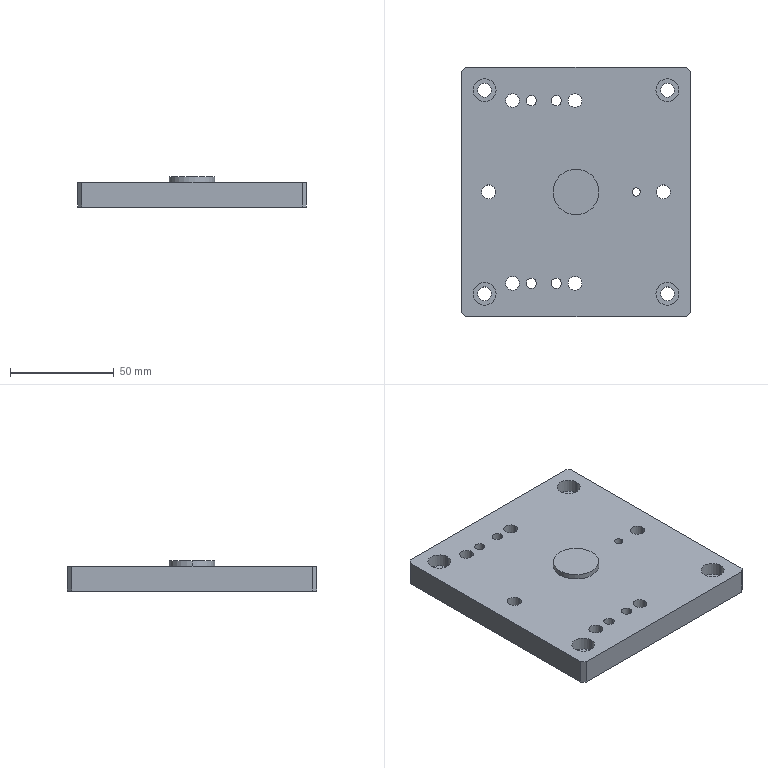Part | STEP file | 11-FG-E02211 | 1 solid | 79 faces | box 110 x 120 x 14.5 mm | volume 149751 mm3 | cylinder 56 | plane 23 | commonest cylinder face diameters 6.6 x16 11 x16 5 x8 15 x8 6.8 x4 4 x2